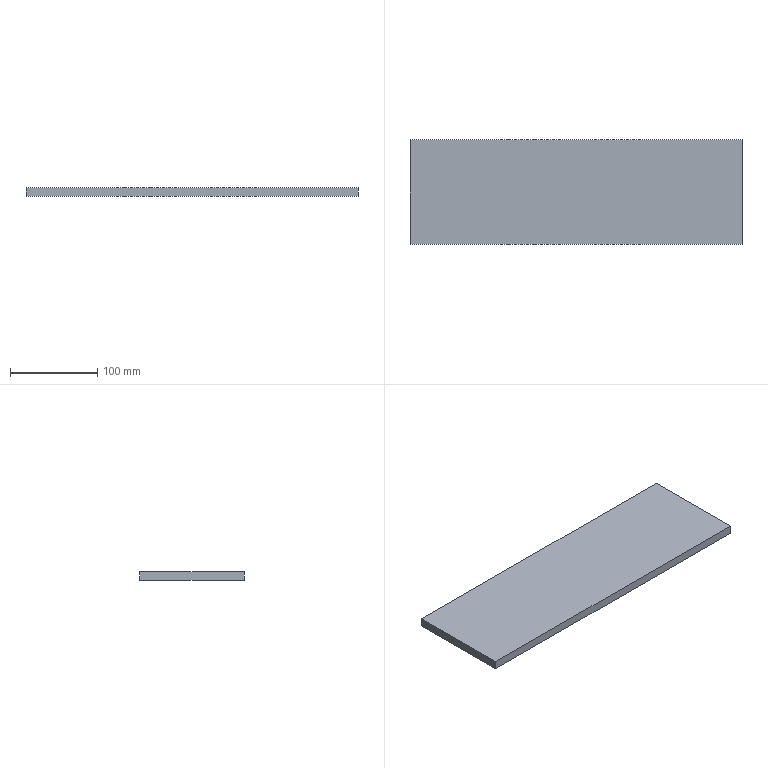Part | NX | features BREP 1 | 1 solid | 6 faces | box 380 x 120 x 10 mm | volume 456000 mm3 | plane 6
STEP:
#1=CARTESIAN_POINT('',(-190.,60.,-5.));
#2=VERTEX_POINT('',#1);
#3=CARTESIAN_POINT('',(-190.,-60.,-5.));
#4=VERTEX_POINT('',#3);
#5=CARTESIAN_POINT('',(-190.,60.,-5.));
#6=DIRECTION('',(0.,-1.,0.));
#7=VECTOR('',#6,1000.);
#8=LINE('',#5,#7);
#9=EDGE_CURVE('',#2,#4,#8,.T.);
#10=ORIENTED_EDGE('',*,*,#9,.T.);
#11=CARTESIAN_POINT('',(-190.,-60.,5.));
#12=VERTEX_POINT('',#11);
#13=CARTESIAN_POINT('',(-190.,-60.,5.));
#14=DIRECTION('',(0.,0.,-1.));
#15=VECTOR('',#14,1000.);
#16=LINE('',#13,#15);
#17=EDGE_CURVE('',#12,#4,#16,.T.);
#18=ORIENTED_EDGE('',*,*,#17,.F.);
#19=CARTESIAN_POINT('',(-190.,60.,5.));
#20=VERTEX_POINT('',#19);
#21=CARTESIAN_POINT('',(-190.,60.,5.));
#22=DIRECTION('',(0.,-1.,0.));
#23=VECTOR('',#22,1000.);
#24=LINE('',#21,#23);
#25=EDGE_CURVE('',#20,#12,#24,.T.);
#26=ORIENTED_EDGE('',*,*,#25,.F.);
#27=CARTESIAN_POINT('',(-190.,60.,5.));
#28=DIRECTION('',(0.,0.,-1.));
#29=VECTOR('',#28,1000.);
#30=LINE('',#27,#29);
#31=EDGE_CURVE('',#20,#2,#30,.T.);
#32=ORIENTED_EDGE('',*,*,#31,.T.);
#33=EDGE_LOOP('',(#10,#18,#26,#32));
#34=FACE_BOUND('',#33,.T.);
#35=CARTESIAN_POINT('',(-190.,60.,5.));
#36=DIRECTION('',(1.,0.,0.));
#37=DIRECTION('',(0.,0.,1.));
#38=AXIS2_PLACEMENT_3D('',#35,#36,#37);
#39=PLANE('',#38);
#40=ADVANCED_FACE('',(#34),#39,.F.);
#41=CARTESIAN_POINT('',(190.,-60.,-5.));
#42=VERTEX_POINT('',#41);
#43=CARTESIAN_POINT('',(-190.,-60.,-5.));
#44=DIRECTION('',(1.,0.,0.));
#45=VECTOR('',#44,1000.);
#46=LINE('',#43,#45);
#47=EDGE_CURVE('',#4,#42,#46,.T.);
#48=ORIENTED_EDGE('',*,*,#47,.T.);
#49=CARTESIAN_POINT('',(190.,-60.,5.));
#50=VERTEX_POINT('',#49);
#51=CARTESIAN_POINT('',(190.,-60.,5.));
#52=DIRECTION('',(0.,0.,-1.));
#53=VECTOR('',#52,1000.);
#54=LINE('',#51,#53);
#55=EDGE_CURVE('',#50,#42,#54,.T.);
#56=ORIENTED_EDGE('',*,*,#55,.F.);
#57=CARTESIAN_POINT('',(-190.,-60.,5.));
#58=DIRECTION('',(1.,0.,0.));
#59=VECTOR('',#58,1000.);
#60=LINE('',#57,#59);
#61=EDGE_CURVE('',#12,#50,#60,.T.);
#62=ORIENTED_EDGE('',*,*,#61,.F.);
#63=ORIENTED_EDGE('',*,*,#17,.T.);
#64=EDGE_LOOP('',(#48,#56,#62,#63));
#65=FACE_BOUND('',#64,.T.);
#66=CARTESIAN_POINT('',(-190.,-60.,5.));
#67=DIRECTION('',(0.,1.,0.));
#68=DIRECTION('',(0.,0.,-1.));
#69=AXIS2_PLACEMENT_3D('',#66,#67,#68);
#70=PLANE('',#69);
#71=ADVANCED_FACE('',(#65),#70,.F.);
#72=CARTESIAN_POINT('',(190.,60.,-5.));
#73=VERTEX_POINT('',#72);
#74=CARTESIAN_POINT('',(190.,60.,-5.));
#75=DIRECTION('',(0.,1.,0.));
#76=VECTOR('',#75,1000.);
#77=LINE('',#74,#76);
#78=EDGE_CURVE('',#42,#73,#77,.T.);
#79=ORIENTED_EDGE('',*,*,#78,.T.);
#80=CARTESIAN_POINT('',(190.,60.,5.));
#81=VERTEX_POINT('',#80);
#82=CARTESIAN_POINT('',(190.,60.,5.));
#83=DIRECTION('',(0.,0.,-1.));
#84=VECTOR('',#83,1000.);
#85=LINE('',#82,#84);
#86=EDGE_CURVE('',#81,#73,#85,.T.);
#87=ORIENTED_EDGE('',*,*,#86,.F.);
#88=CARTESIAN_POINT('',(190.,60.,5.));
#89=DIRECTION('',(0.,1.,0.));
#90=VECTOR('',#89,1000.);
#91=LINE('',#88,#90);
#92=EDGE_CURVE('',#50,#81,#91,.T.);
#93=ORIENTED_EDGE('',*,*,#92,.F.);
#94=ORIENTED_EDGE('',*,*,#55,.T.);
#95=EDGE_LOOP('',(#79,#87,#93,#94));
#96=FACE_BOUND('',#95,.T.);
#97=CARTESIAN_POINT('',(190.,60.,5.));
#98=DIRECTION('',(-1.,0.,0.));
#99=DIRECTION('',(0.,0.,-1.));
#100=AXIS2_PLACEMENT_3D('',#97,#98,#99);
#101=PLANE('',#100);
#102=ADVANCED_FACE('',(#96),#101,.F.);
#103=CARTESIAN_POINT('',(-190.,60.,-5.));
#104=DIRECTION('',(-1.,0.,0.));
#105=VECTOR('',#104,1000.);
#106=LINE('',#103,#105);
#107=EDGE_CURVE('',#73,#2,#106,.T.);
#108=ORIENTED_EDGE('',*,*,#107,.T.);
#109=ORIENTED_EDGE('',*,*,#31,.F.);
#110=CARTESIAN_POINT('',(-190.,60.,5.));
#111=DIRECTION('',(-1.,0.,0.));
#112=VECTOR('',#111,1000.);
#113=LINE('',#110,#112);
#114=EDGE_CURVE('',#81,#20,#113,.T.);
#115=ORIENTED_EDGE('',*,*,#114,.F.);
#116=ORIENTED_EDGE('',*,*,#86,.T.);
#117=EDGE_LOOP('',(#108,#109,#115,#116));
#118=FACE_BOUND('',#117,.T.);
#119=CARTESIAN_POINT('',(-190.,60.,5.));
#120=DIRECTION('',(0.,-1.,0.));
#121=DIRECTION('',(0.,0.,1.));
#122=AXIS2_PLACEMENT_3D('',#119,#120,#121);
#123=PLANE('',#122);
#124=ADVANCED_FACE('',(#118),#123,.F.);
#125=ORIENTED_EDGE('',*,*,#25,.T.);
#126=ORIENTED_EDGE('',*,*,#61,.T.);
#127=ORIENTED_EDGE('',*,*,#92,.T.);
#128=ORIENTED_EDGE('',*,*,#114,.T.);
#129=EDGE_LOOP('',(#125,#126,#127,#128));
#130=FACE_BOUND('',#129,.T.);
#131=CARTESIAN_POINT('',(-190.,-60.,5.));
#132=DIRECTION('',(0.,0.,1.));
#133=DIRECTION('',(-1.,0.,0.));
#134=AXIS2_PLACEMENT_3D('',#131,#132,#133);
#135=PLANE('',#134);
#136=ADVANCED_FACE('',(#130),#135,.T.);
#137=ORIENTED_EDGE('',*,*,#9,.F.);
#138=ORIENTED_EDGE('',*,*,#107,.F.);
#139=ORIENTED_EDGE('',*,*,#78,.F.);
#140=ORIENTED_EDGE('',*,*,#47,.F.);
#141=EDGE_LOOP('',(#137,#138,#139,#140));
#142=FACE_BOUND('',#141,.T.);
#143=CARTESIAN_POINT('',(-190.,-60.,-5.));
#144=DIRECTION('',(0.,0.,1.));
#145=DIRECTION('',(-1.,0.,0.));
#146=AXIS2_PLACEMENT_3D('',#143,#144,#145);
#147=PLANE('',#146);
#148=ADVANCED_FACE('',(#142),#147,.F.);
#149=CLOSED_SHELL('',(#40,#71,#102,#124,#136,#148));
#150=MANIFOLD_SOLID_BREP('',#149);
#151=(LENGTH_UNIT()NAMED_UNIT(*)SI_UNIT(.MILLI.,.METRE.));
#152=UNCERTAINTY_MEASURE_WITH_UNIT(LENGTH_MEASURE(0.00001),#151,'','');
#153=(NAMED_UNIT(*)PLANE_ANGLE_UNIT()SI_UNIT($,.RADIAN.));
#154=(NAMED_UNIT(*)SI_UNIT($,.STERADIAN.)SOLID_ANGLE_UNIT());
#155=(GEOMETRIC_REPRESENTATION_CONTEXT(3)GLOBAL_UNCERTAINTY_ASSIGNED_CONTEXT((#152))GLOBAL_UNIT_ASSIGNED_CONTEXT((#151,#153,#154))REPRESENTATION_CONTEXT('',''));
#156=ADVANCED_BREP_SHAPE_REPRESENTATION('',(#150),#155);